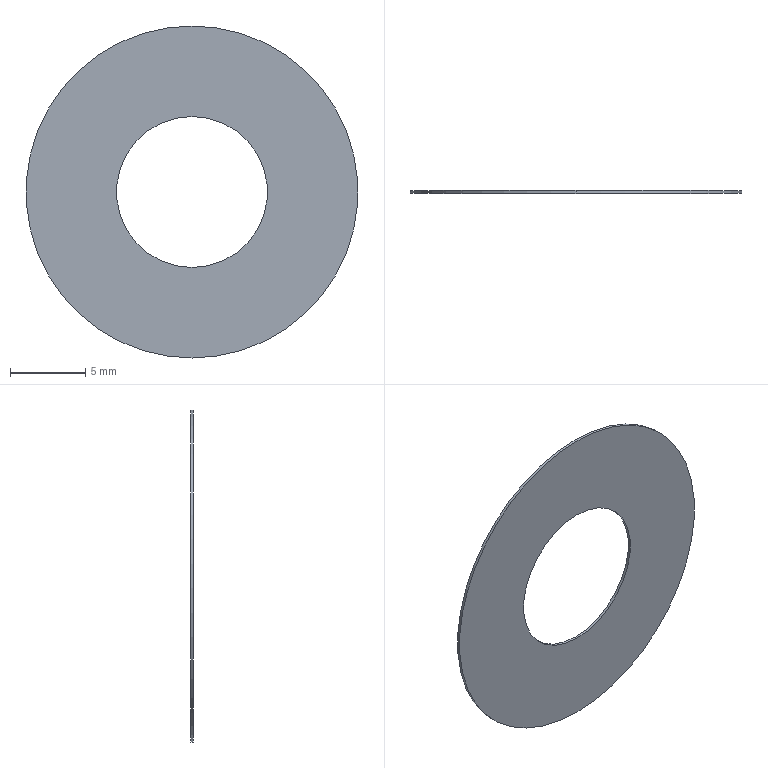Part | SolidWorks | features BaseBody 1 | 1 solid | 6 faces | box 22 x 0.18 x 22 mm | volume 54.287 mm3 | cylinder 4 | plane 2 | commonest cylinder face diameters 10 x2 22 x2
STEP:
#1=CARTESIAN_POINT('',(0.,0.18,5.));
#2=VERTEX_POINT('',#1);
#3=CARTESIAN_POINT('',(0.,0.,5.));
#4=VERTEX_POINT('',#3);
#5=CARTESIAN_POINT('',(0.,0.18,5.));
#6=DIRECTION('',(0.,-1.,0.));
#7=VECTOR('',#6,1000.);
#8=LINE('',#5,#7);
#9=EDGE_CURVE('',#2,#4,#8,.T.);
#10=ORIENTED_EDGE('',*,*,#9,.F.);
#11=CARTESIAN_POINT('',(0.,0.18,-5.));
#12=VERTEX_POINT('',#11);
#13=CARTESIAN_POINT('',(0.,0.18,0.));
#14=DIRECTION('',(0.,1.,0.));
#15=DIRECTION('',(0.,0.,1.));
#16=AXIS2_PLACEMENT_3D('',#13,#14,#15);
#17=CIRCLE('',#16,5.);
#18=EDGE_CURVE('',#2,#12,#17,.T.);
#19=ORIENTED_EDGE('',*,*,#18,.T.);
#20=CARTESIAN_POINT('',(0.,0.,-5.));
#21=VERTEX_POINT('',#20);
#22=CARTESIAN_POINT('',(0.,0.18,-5.));
#23=DIRECTION('',(0.,-1.,0.));
#24=VECTOR('',#23,1000.);
#25=LINE('',#22,#24);
#26=EDGE_CURVE('',#12,#21,#25,.T.);
#27=ORIENTED_EDGE('',*,*,#26,.T.);
#28=CARTESIAN_POINT('',(0.,0.,0.));
#29=DIRECTION('',(0.,1.,0.));
#30=DIRECTION('',(0.,0.,1.));
#31=AXIS2_PLACEMENT_3D('',#28,#29,#30);
#32=CIRCLE('',#31,5.);
#33=EDGE_CURVE('',#4,#21,#32,.T.);
#34=ORIENTED_EDGE('',*,*,#33,.F.);
#35=EDGE_LOOP('',(#10,#19,#27,#34));
#36=FACE_OUTER_BOUND('',#35,.T.);
#37=CARTESIAN_POINT('',(0.,0.18,0.));
#38=DIRECTION('',(0.,-1.,0.));
#39=DIRECTION('',(0.,0.,-1.));
#40=AXIS2_PLACEMENT_3D('',#37,#38,#39);
#41=CYLINDRICAL_SURFACE('',#40,5.);
#42=ADVANCED_FACE('',(#36),#41,.F.);
#43=CARTESIAN_POINT('',(0.,0.18,11.));
#44=VERTEX_POINT('',#43);
#45=CARTESIAN_POINT('',(0.,0.,11.));
#46=VERTEX_POINT('',#45);
#47=CARTESIAN_POINT('',(0.,0.18,11.));
#48=DIRECTION('',(0.,-1.,0.));
#49=VECTOR('',#48,1000.);
#50=LINE('',#47,#49);
#51=EDGE_CURVE('',#44,#46,#50,.T.);
#52=ORIENTED_EDGE('',*,*,#51,.F.);
#53=CARTESIAN_POINT('',(0.,0.18,-11.));
#54=VERTEX_POINT('',#53);
#55=CARTESIAN_POINT('',(0.,0.18,0.));
#56=DIRECTION('',(0.,1.,0.));
#57=DIRECTION('',(0.,0.,1.));
#58=AXIS2_PLACEMENT_3D('',#55,#56,#57);
#59=CIRCLE('',#58,11.);
#60=EDGE_CURVE('',#54,#44,#59,.T.);
#61=ORIENTED_EDGE('',*,*,#60,.F.);
#62=CARTESIAN_POINT('',(0.,0.,-11.));
#63=VERTEX_POINT('',#62);
#64=CARTESIAN_POINT('',(0.,0.18,-11.));
#65=DIRECTION('',(0.,-1.,0.));
#66=VECTOR('',#65,1000.);
#67=LINE('',#64,#66);
#68=EDGE_CURVE('',#54,#63,#67,.T.);
#69=ORIENTED_EDGE('',*,*,#68,.T.);
#70=CARTESIAN_POINT('',(0.,0.,0.));
#71=DIRECTION('',(0.,1.,0.));
#72=DIRECTION('',(0.,0.,1.));
#73=AXIS2_PLACEMENT_3D('',#70,#71,#72);
#74=CIRCLE('',#73,11.);
#75=EDGE_CURVE('',#63,#46,#74,.T.);
#76=ORIENTED_EDGE('',*,*,#75,.T.);
#77=EDGE_LOOP('',(#52,#61,#69,#76));
#78=FACE_OUTER_BOUND('',#77,.T.);
#79=CARTESIAN_POINT('',(0.,0.18,0.));
#80=DIRECTION('',(0.,-1.,0.));
#81=DIRECTION('',(0.,0.,-1.));
#82=AXIS2_PLACEMENT_3D('',#79,#80,#81);
#83=CYLINDRICAL_SURFACE('',#82,11.);
#84=ADVANCED_FACE('',(#78),#83,.T.);
#85=CARTESIAN_POINT('',(0.,0.,0.));
#86=DIRECTION('',(0.,1.,0.));
#87=DIRECTION('',(0.,0.,1.));
#88=AXIS2_PLACEMENT_3D('',#85,#86,#87);
#89=CIRCLE('',#88,5.);
#90=EDGE_CURVE('',#21,#4,#89,.T.);
#91=ORIENTED_EDGE('',*,*,#90,.T.);
#92=ORIENTED_EDGE('',*,*,#33,.T.);
#93=EDGE_LOOP('',(#91,#92));
#94=FACE_BOUND('',#93,.T.);
#95=ORIENTED_EDGE('',*,*,#75,.F.);
#96=CARTESIAN_POINT('',(0.,0.,0.));
#97=DIRECTION('',(0.,1.,0.));
#98=DIRECTION('',(0.,0.,1.));
#99=AXIS2_PLACEMENT_3D('',#96,#97,#98);
#100=CIRCLE('',#99,11.);
#101=EDGE_CURVE('',#46,#63,#100,.T.);
#102=ORIENTED_EDGE('',*,*,#101,.F.);
#103=EDGE_LOOP('',(#95,#102));
#104=FACE_OUTER_BOUND('',#103,.T.);
#105=CARTESIAN_POINT('',(0.,0.,0.));
#106=DIRECTION('',(0.,1.,0.));
#107=DIRECTION('',(1.,0.,0.));
#108=AXIS2_PLACEMENT_3D('',#105,#106,#107);
#109=PLANE('',#108);
#110=ADVANCED_FACE('',(#94,#104),#109,.F.);
#111=CARTESIAN_POINT('',(0.,0.18,0.));
#112=DIRECTION('',(0.,1.,0.));
#113=DIRECTION('',(0.,0.,1.));
#114=AXIS2_PLACEMENT_3D('',#111,#112,#113);
#115=CIRCLE('',#114,5.);
#116=EDGE_CURVE('',#12,#2,#115,.T.);
#117=ORIENTED_EDGE('',*,*,#116,.F.);
#118=ORIENTED_EDGE('',*,*,#18,.F.);
#119=EDGE_LOOP('',(#117,#118));
#120=FACE_BOUND('',#119,.T.);
#121=ORIENTED_EDGE('',*,*,#60,.T.);
#122=CARTESIAN_POINT('',(0.,0.18,0.));
#123=DIRECTION('',(0.,1.,0.));
#124=DIRECTION('',(0.,0.,1.));
#125=AXIS2_PLACEMENT_3D('',#122,#123,#124);
#126=CIRCLE('',#125,11.);
#127=EDGE_CURVE('',#44,#54,#126,.T.);
#128=ORIENTED_EDGE('',*,*,#127,.T.);
#129=EDGE_LOOP('',(#121,#128));
#130=FACE_OUTER_BOUND('',#129,.T.);
#131=CARTESIAN_POINT('',(0.,0.18,0.));
#132=DIRECTION('',(0.,1.,0.));
#133=DIRECTION('',(1.,0.,0.));
#134=AXIS2_PLACEMENT_3D('',#131,#132,#133);
#135=PLANE('',#134);
#136=ADVANCED_FACE('',(#120,#130),#135,.T.);
#137=ORIENTED_EDGE('',*,*,#127,.F.);
#138=ORIENTED_EDGE('',*,*,#51,.T.);
#139=ORIENTED_EDGE('',*,*,#101,.T.);
#140=ORIENTED_EDGE('',*,*,#68,.F.);
#141=EDGE_LOOP('',(#137,#138,#139,#140));
#142=FACE_OUTER_BOUND('',#141,.T.);
#143=CARTESIAN_POINT('',(0.,0.18,0.));
#144=DIRECTION('',(0.,-1.,0.));
#145=DIRECTION('',(0.,0.,-1.));
#146=AXIS2_PLACEMENT_3D('',#143,#144,#145);
#147=CYLINDRICAL_SURFACE('',#146,11.);
#148=ADVANCED_FACE('',(#142),#147,.T.);
#149=ORIENTED_EDGE('',*,*,#116,.T.);
#150=ORIENTED_EDGE('',*,*,#9,.T.);
#151=ORIENTED_EDGE('',*,*,#90,.F.);
#152=ORIENTED_EDGE('',*,*,#26,.F.);
#153=EDGE_LOOP('',(#149,#150,#151,#152));
#154=FACE_OUTER_BOUND('',#153,.T.);
#155=CARTESIAN_POINT('',(0.,0.18,0.));
#156=DIRECTION('',(0.,-1.,0.));
#157=DIRECTION('',(0.,0.,-1.));
#158=AXIS2_PLACEMENT_3D('',#155,#156,#157);
#159=CYLINDRICAL_SURFACE('',#158,5.);
#160=ADVANCED_FACE('',(#154),#159,.F.);
#161=CLOSED_SHELL('',(#42,#84,#110,#136,#148,#160));
#162=MANIFOLD_SOLID_BREP('',#161);
#163=CARTESIAN_POINT('',(0.,0.,0.));
#164=DIRECTION('',(0.,0.,1.));
#165=DIRECTION('',(1.,0.,0.));
#166=AXIS2_PLACEMENT_3D('',#163,#164,#165);
#167=(LENGTH_UNIT()NAMED_UNIT(*)SI_UNIT(.MILLI.,.METRE.));
#168=UNCERTAINTY_MEASURE_WITH_UNIT(LENGTH_MEASURE(0.00001),#167,'','');
#169=(NAMED_UNIT(*)PLANE_ANGLE_UNIT()SI_UNIT($,.RADIAN.));
#170=(NAMED_UNIT(*)SI_UNIT($,.STERADIAN.)SOLID_ANGLE_UNIT());
#171=(GEOMETRIC_REPRESENTATION_CONTEXT(3)GLOBAL_UNCERTAINTY_ASSIGNED_CONTEXT((#168))GLOBAL_UNIT_ASSIGNED_CONTEXT((#167,#169,#170))REPRESENTATION_CONTEXT('',''));
#172=ADVANCED_BREP_SHAPE_REPRESENTATION('',(#162,#166),#171);